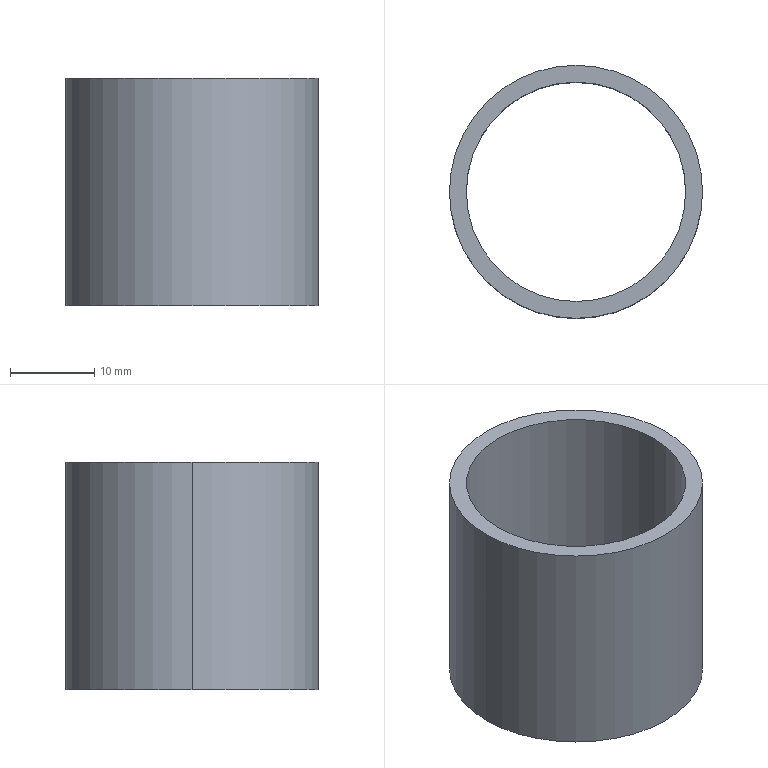Part | SolidWorks | features Extrusion 1 | 1 solid | 6 faces | box 30 x 30 x 27 mm | volume 4750 mm3 | cylinder 4 | plane 2 | commonest cylinder face diameters 26 x2 30 x2
STEP:
#1=CARTESIAN_POINT('',(-13.,0.,27.));
#2=VERTEX_POINT('',#1);
#3=CARTESIAN_POINT('',(13.,0.,27.));
#4=VERTEX_POINT('',#3);
#5=CARTESIAN_POINT('',(0.,0.,27.));
#6=DIRECTION('',(0.,0.,1.));
#7=DIRECTION('',(1.,0.,0.));
#8=AXIS2_PLACEMENT_3D('',#5,#6,#7);
#9=CIRCLE('',#8,13.);
#10=EDGE_CURVE('',#2,#4,#9,.T.);
#11=ORIENTED_EDGE('',*,*,#10,.T.);
#12=CARTESIAN_POINT('',(13.,0.,0.));
#13=VERTEX_POINT('',#12);
#14=CARTESIAN_POINT('',(13.,0.,27.));
#15=DIRECTION('',(0.,0.,-1.));
#16=VECTOR('',#15,1000.);
#17=LINE('',#14,#16);
#18=EDGE_CURVE('',#4,#13,#17,.T.);
#19=ORIENTED_EDGE('',*,*,#18,.T.);
#20=CARTESIAN_POINT('',(-13.,0.,0.));
#21=VERTEX_POINT('',#20);
#22=CARTESIAN_POINT('',(0.,0.,0.));
#23=DIRECTION('',(0.,0.,1.));
#24=DIRECTION('',(1.,0.,0.));
#25=AXIS2_PLACEMENT_3D('',#22,#23,#24);
#26=CIRCLE('',#25,13.);
#27=EDGE_CURVE('',#21,#13,#26,.T.);
#28=ORIENTED_EDGE('',*,*,#27,.F.);
#29=CARTESIAN_POINT('',(-13.,0.,27.));
#30=DIRECTION('',(0.,0.,-1.));
#31=VECTOR('',#30,1000.);
#32=LINE('',#29,#31);
#33=EDGE_CURVE('',#2,#21,#32,.T.);
#34=ORIENTED_EDGE('',*,*,#33,.F.);
#35=EDGE_LOOP('',(#11,#19,#28,#34));
#36=FACE_OUTER_BOUND('',#35,.T.);
#37=CARTESIAN_POINT('',(0.,0.,27.));
#38=DIRECTION('',(0.,0.,-1.));
#39=DIRECTION('',(-1.,0.,0.));
#40=AXIS2_PLACEMENT_3D('',#37,#38,#39);
#41=CYLINDRICAL_SURFACE('',#40,13.);
#42=ADVANCED_FACE('',(#36),#41,.F.);
#43=CARTESIAN_POINT('',(15.,0.,27.));
#44=VERTEX_POINT('',#43);
#45=CARTESIAN_POINT('',(-15.,0.,27.));
#46=VERTEX_POINT('',#45);
#47=CARTESIAN_POINT('',(0.,0.,27.));
#48=DIRECTION('',(0.,0.,1.));
#49=DIRECTION('',(1.,0.,0.));
#50=AXIS2_PLACEMENT_3D('',#47,#48,#49);
#51=CIRCLE('',#50,15.);
#52=EDGE_CURVE('',#44,#46,#51,.T.);
#53=ORIENTED_EDGE('',*,*,#52,.F.);
#54=CARTESIAN_POINT('',(15.,0.,0.));
#55=VERTEX_POINT('',#54);
#56=CARTESIAN_POINT('',(15.,0.,27.));
#57=DIRECTION('',(0.,0.,-1.));
#58=VECTOR('',#57,1000.);
#59=LINE('',#56,#58);
#60=EDGE_CURVE('',#44,#55,#59,.T.);
#61=ORIENTED_EDGE('',*,*,#60,.T.);
#62=CARTESIAN_POINT('',(-15.,0.,0.));
#63=VERTEX_POINT('',#62);
#64=CARTESIAN_POINT('',(0.,0.,0.));
#65=DIRECTION('',(0.,0.,1.));
#66=DIRECTION('',(1.,0.,0.));
#67=AXIS2_PLACEMENT_3D('',#64,#65,#66);
#68=CIRCLE('',#67,15.);
#69=EDGE_CURVE('',#55,#63,#68,.T.);
#70=ORIENTED_EDGE('',*,*,#69,.T.);
#71=CARTESIAN_POINT('',(-15.,0.,27.));
#72=DIRECTION('',(0.,0.,-1.));
#73=VECTOR('',#72,1000.);
#74=LINE('',#71,#73);
#75=EDGE_CURVE('',#46,#63,#74,.T.);
#76=ORIENTED_EDGE('',*,*,#75,.F.);
#77=EDGE_LOOP('',(#53,#61,#70,#76));
#78=FACE_OUTER_BOUND('',#77,.T.);
#79=CARTESIAN_POINT('',(0.,0.,27.));
#80=DIRECTION('',(0.,0.,-1.));
#81=DIRECTION('',(-1.,0.,0.));
#82=AXIS2_PLACEMENT_3D('',#79,#80,#81);
#83=CYLINDRICAL_SURFACE('',#82,15.);
#84=ADVANCED_FACE('',(#78),#83,.T.);
#85=CARTESIAN_POINT('',(0.,0.,27.));
#86=DIRECTION('',(0.,0.,1.));
#87=DIRECTION('',(1.,0.,0.));
#88=AXIS2_PLACEMENT_3D('',#85,#86,#87);
#89=CIRCLE('',#88,15.);
#90=EDGE_CURVE('',#46,#44,#89,.T.);
#91=ORIENTED_EDGE('',*,*,#90,.T.);
#92=ORIENTED_EDGE('',*,*,#52,.T.);
#93=EDGE_LOOP('',(#91,#92));
#94=FACE_OUTER_BOUND('',#93,.T.);
#95=ORIENTED_EDGE('',*,*,#10,.F.);
#96=CARTESIAN_POINT('',(0.,0.,27.));
#97=DIRECTION('',(0.,0.,1.));
#98=DIRECTION('',(1.,0.,0.));
#99=AXIS2_PLACEMENT_3D('',#96,#97,#98);
#100=CIRCLE('',#99,13.);
#101=EDGE_CURVE('',#4,#2,#100,.T.);
#102=ORIENTED_EDGE('',*,*,#101,.F.);
#103=EDGE_LOOP('',(#95,#102));
#104=FACE_BOUND('',#103,.T.);
#105=CARTESIAN_POINT('',(0.,0.,27.));
#106=DIRECTION('',(0.,0.,1.));
#107=DIRECTION('',(1.,0.,0.));
#108=AXIS2_PLACEMENT_3D('',#105,#106,#107);
#109=PLANE('',#108);
#110=ADVANCED_FACE('',(#94,#104),#109,.T.);
#111=CARTESIAN_POINT('',(0.,0.,0.));
#112=DIRECTION('',(0.,0.,1.));
#113=DIRECTION('',(1.,0.,0.));
#114=AXIS2_PLACEMENT_3D('',#111,#112,#113);
#115=CIRCLE('',#114,15.);
#116=EDGE_CURVE('',#63,#55,#115,.T.);
#117=ORIENTED_EDGE('',*,*,#116,.F.);
#118=ORIENTED_EDGE('',*,*,#69,.F.);
#119=EDGE_LOOP('',(#117,#118));
#120=FACE_OUTER_BOUND('',#119,.T.);
#121=ORIENTED_EDGE('',*,*,#27,.T.);
#122=CARTESIAN_POINT('',(0.,0.,0.));
#123=DIRECTION('',(0.,0.,1.));
#124=DIRECTION('',(1.,0.,0.));
#125=AXIS2_PLACEMENT_3D('',#122,#123,#124);
#126=CIRCLE('',#125,13.);
#127=EDGE_CURVE('',#13,#21,#126,.T.);
#128=ORIENTED_EDGE('',*,*,#127,.T.);
#129=EDGE_LOOP('',(#121,#128));
#130=FACE_BOUND('',#129,.T.);
#131=CARTESIAN_POINT('',(0.,0.,0.));
#132=DIRECTION('',(0.,0.,1.));
#133=DIRECTION('',(1.,0.,0.));
#134=AXIS2_PLACEMENT_3D('',#131,#132,#133);
#135=PLANE('',#134);
#136=ADVANCED_FACE('',(#120,#130),#135,.F.);
#137=ORIENTED_EDGE('',*,*,#60,.F.);
#138=ORIENTED_EDGE('',*,*,#90,.F.);
#139=ORIENTED_EDGE('',*,*,#75,.T.);
#140=ORIENTED_EDGE('',*,*,#116,.T.);
#141=EDGE_LOOP('',(#137,#138,#139,#140));
#142=FACE_OUTER_BOUND('',#141,.T.);
#143=CARTESIAN_POINT('',(0.,0.,27.));
#144=DIRECTION('',(0.,0.,-1.));
#145=DIRECTION('',(-1.,0.,0.));
#146=AXIS2_PLACEMENT_3D('',#143,#144,#145);
#147=CYLINDRICAL_SURFACE('',#146,15.);
#148=ADVANCED_FACE('',(#142),#147,.T.);
#149=ORIENTED_EDGE('',*,*,#18,.F.);
#150=ORIENTED_EDGE('',*,*,#101,.T.);
#151=ORIENTED_EDGE('',*,*,#33,.T.);
#152=ORIENTED_EDGE('',*,*,#127,.F.);
#153=EDGE_LOOP('',(#149,#150,#151,#152));
#154=FACE_OUTER_BOUND('',#153,.T.);
#155=CARTESIAN_POINT('',(0.,0.,27.));
#156=DIRECTION('',(0.,0.,-1.));
#157=DIRECTION('',(-1.,0.,0.));
#158=AXIS2_PLACEMENT_3D('',#155,#156,#157);
#159=CYLINDRICAL_SURFACE('',#158,13.);
#160=ADVANCED_FACE('',(#154),#159,.F.);
#161=CLOSED_SHELL('',(#42,#84,#110,#136,#148,#160));
#162=MANIFOLD_SOLID_BREP('',#161);
#163=CARTESIAN_POINT('',(0.,0.,0.));
#164=DIRECTION('',(0.,0.,1.));
#165=DIRECTION('',(1.,0.,0.));
#166=AXIS2_PLACEMENT_3D('',#163,#164,#165);
#167=(LENGTH_UNIT()NAMED_UNIT(*)SI_UNIT(.MILLI.,.METRE.));
#168=UNCERTAINTY_MEASURE_WITH_UNIT(LENGTH_MEASURE(0.00001),#167,'','');
#169=(NAMED_UNIT(*)PLANE_ANGLE_UNIT()SI_UNIT($,.RADIAN.));
#170=(NAMED_UNIT(*)SI_UNIT($,.STERADIAN.)SOLID_ANGLE_UNIT());
#171=(GEOMETRIC_REPRESENTATION_CONTEXT(3)GLOBAL_UNCERTAINTY_ASSIGNED_CONTEXT((#168))GLOBAL_UNIT_ASSIGNED_CONTEXT((#167,#169,#170))REPRESENTATION_CONTEXT('',''));
#172=ADVANCED_BREP_SHAPE_REPRESENTATION('',(#162,#166),#171);